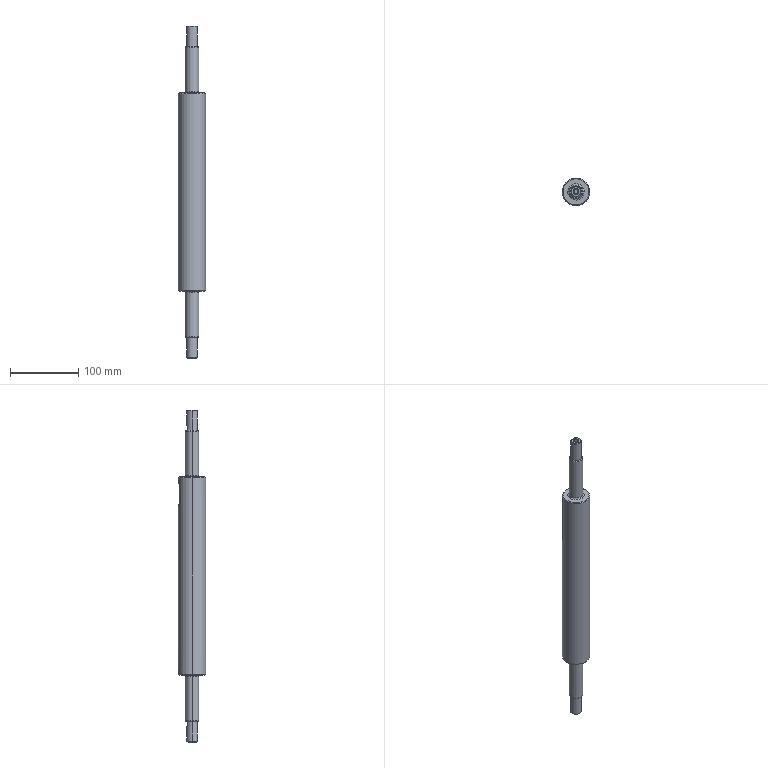Part | STEP file | Synchronous shaft 2 | 1 solid | 57 faces | box 40 x 40 x 486 mm | volume 415215 mm3 | cylinder 20 | plane 17 | cone 16 | spline 4 | commonest cylinder face diameters 6 x4 16 x4 20 x4 5 x3 12 x3 40 x2